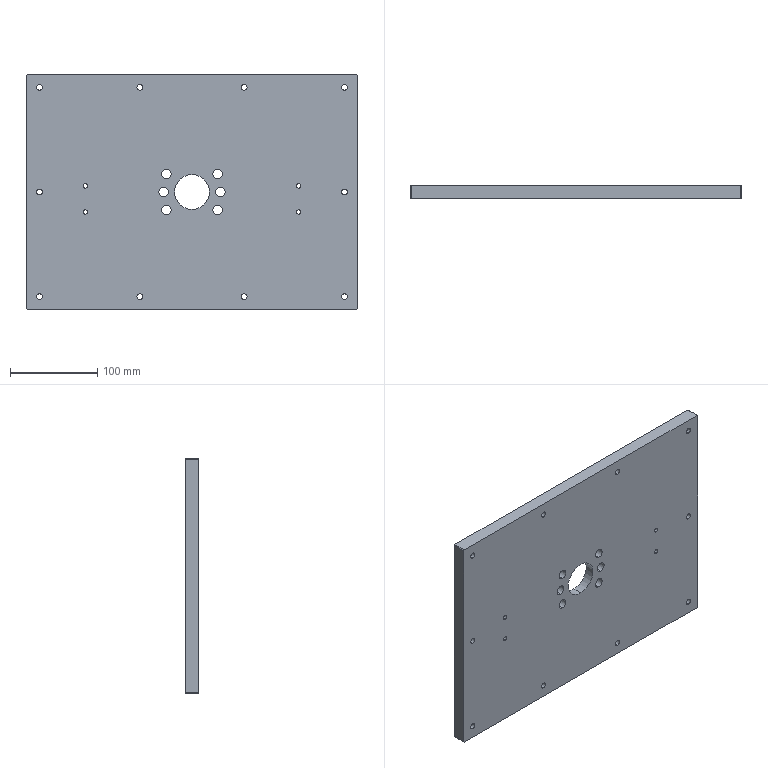Part | SolidWorks | features ICE 4, HoleWzd 2, Chamfer 1, Extrusion 1 | 1 solid | 88 faces | box 380 x 15 x 270 mm | volume 1473539 mm3 | cylinder 66 | plane 22 | commonest cylinder face diameters 11 x32 6.6 x20 5 x8 6 x2 40 x2 105 x2